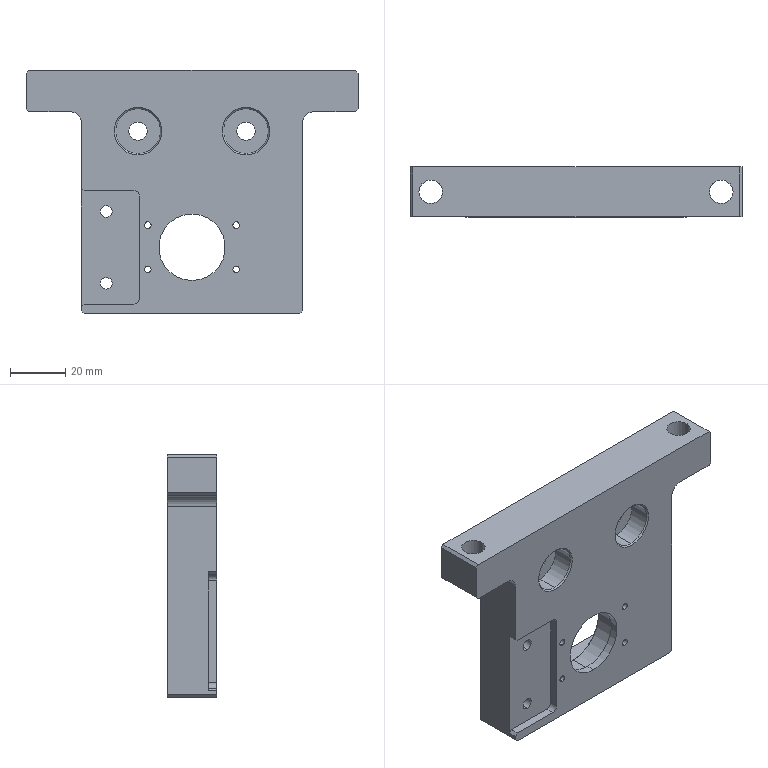Part | STEP file | PN_0001 Lead Screw Support Block Left | 1 solid | 80 faces | box 120 x 18 x 88 mm | volume 113336 mm3 | cylinder 42 | plane 32 | cone 6 | commonest cylinder face diameters 2.4 x8 4 x6 4.2 x4 6.6 x4 8.5 x4 13 x4